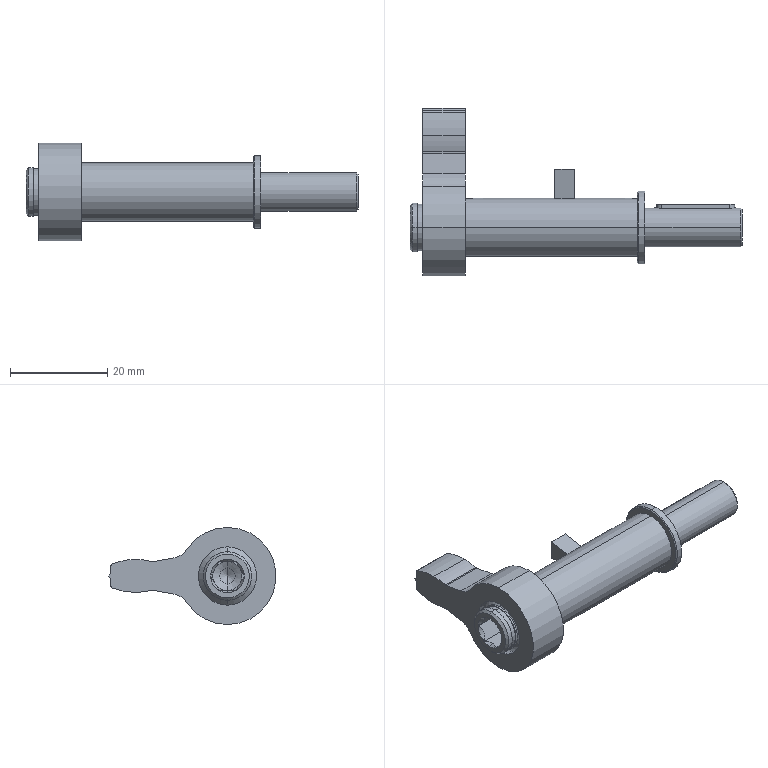Part | STEP file | PN_0052 | 1 solid | 89 faces | box 68.3 x 34.5 x 20 mm | volume 8759 mm3 | cylinder 36 | plane 33 | cone 20 | commonest cylinder face diameters 2 x5 8 x4 10 x4 12 x4 20 x3 26 x3